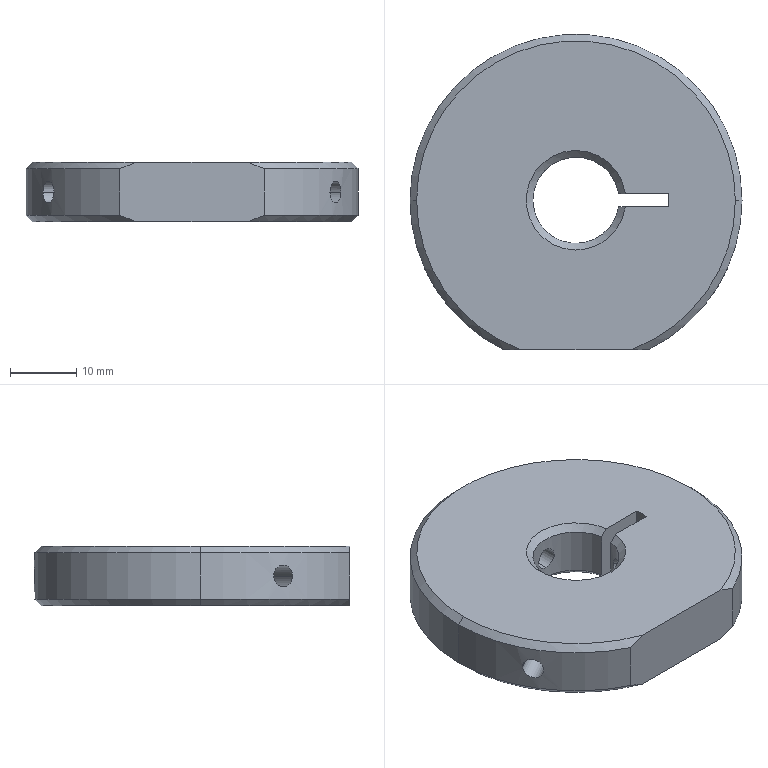Part | STEP file | 11-FG-B05911 | 1 solid | 26 faces | box 50 x 47.5 x 9 mm | volume 15360 mm3 | cylinder 12 | cone 9 | plane 5 | commonest cylinder face diameters 3.3 x6 50 x3 13 x2 28 x1
STEP:
#1=CARTESIAN_POINT('',(24.,0.,9.));
#2=VERTEX_POINT('',#1);
#3=CARTESIAN_POINT('',(-24.,0.,9.));
#4=VERTEX_POINT('',#3);
#5=CARTESIAN_POINT('',(0.,0.,9.));
#6=DIRECTION('',(0.,0.,1.));
#7=DIRECTION('',(1.,0.,0.));
#8=AXIS2_PLACEMENT_3D('',#5,#6,#7);
#9=CIRCLE('',#8,24.);
#10=EDGE_CURVE('',#2,#4,#9,.T.);
#11=ORIENTED_EDGE('',*,*,#10,.F.);
#12=CARTESIAN_POINT('',(25.,0.,8.));
#13=VERTEX_POINT('',#12);
#14=CARTESIAN_POINT('',(24.,0.,9.));
#15=DIRECTION('',(0.7071,0.,-0.7071));
#16=VECTOR('',#15,1000.);
#17=LINE('',#14,#16);
#18=EDGE_CURVE('',#2,#13,#17,.T.);
#19=ORIENTED_EDGE('',*,*,#18,.T.);
#20=CARTESIAN_POINT('',(-25.,0.,8.));
#21=VERTEX_POINT('',#20);
#22=CARTESIAN_POINT('',(0.,0.,8.));
#23=DIRECTION('',(0.,0.,-1.));
#24=DIRECTION('',(1.,0.,0.));
#25=AXIS2_PLACEMENT_3D('',#22,#23,#24);
#26=CIRCLE('',#25,25.);
#27=EDGE_CURVE('',#21,#13,#26,.T.);
#28=ORIENTED_EDGE('',*,*,#27,.F.);
#29=CARTESIAN_POINT('',(-24.,0.,9.));
#30=DIRECTION('',(-0.7071,0.,-0.7071));
#31=VECTOR('',#30,1000.);
#32=LINE('',#29,#31);
#33=EDGE_CURVE('',#4,#21,#32,.T.);
#34=ORIENTED_EDGE('',*,*,#33,.F.);
#35=EDGE_LOOP('',(#11,#19,#28,#34));
#36=FACE_OUTER_BOUND('',#35,.T.);
#37=CARTESIAN_POINT('',(0.,0.,9.));
#38=DIRECTION('',(0.,0.,-1.));
#39=DIRECTION('',(-1.,0.,0.));
#40=AXIS2_PLACEMENT_3D('',#37,#38,#39);
#41=CONICAL_SURFACE('',#40,24.,0.7854);
#42=ADVANCED_FACE('',(#36),#41,.T.);
#43=CARTESIAN_POINT('',(-8.352,-22.5,9.));
#44=VERTEX_POINT('',#43);
#45=CARTESIAN_POINT('',(0.,0.,9.));
#46=DIRECTION('',(0.,0.,1.));
#47=DIRECTION('',(1.,0.,0.));
#48=AXIS2_PLACEMENT_3D('',#45,#46,#47);
#49=CIRCLE('',#48,24.);
#50=EDGE_CURVE('',#4,#44,#49,.T.);
#51=ORIENTED_EDGE('',*,*,#50,.F.);
#52=ORIENTED_EDGE('',*,*,#33,.T.);
#53=CARTESIAN_POINT('',(-10.897,-22.5,8.));
#54=VERTEX_POINT('',#53);
#55=CARTESIAN_POINT('',(0.,0.,8.));
#56=DIRECTION('',(0.,0.,-1.));
#57=DIRECTION('',(1.,0.,0.));
#58=AXIS2_PLACEMENT_3D('',#55,#56,#57);
#59=CIRCLE('',#58,25.);
#60=EDGE_CURVE('',#54,#21,#59,.T.);
#61=ORIENTED_EDGE('',*,*,#60,.F.);
#62=CARTESIAN_POINT('',(-8.352,-22.5,9.));
#63=CARTESIAN_POINT('',(-9.21,-22.5,8.701));
#64=CARTESIAN_POINT('',(-10.062,-22.5,8.364));
#65=CARTESIAN_POINT('',(-10.897,-22.5,8.));
#66=B_SPLINE_CURVE_WITH_KNOTS('',3,(#62,#63,#64,#65),.UNSPECIFIED.,.F.,.F.,(4,4),(0.06645,0.06918),.UNSPECIFIED.);
#67=EDGE_CURVE('',#44,#54,#66,.T.);
#68=ORIENTED_EDGE('',*,*,#67,.F.);
#69=EDGE_LOOP('',(#51,#52,#61,#68));
#70=FACE_OUTER_BOUND('',#69,.T.);
#71=CARTESIAN_POINT('',(0.,0.,9.));
#72=DIRECTION('',(0.,0.,-1.));
#73=DIRECTION('',(-1.,0.,0.));
#74=AXIS2_PLACEMENT_3D('',#71,#72,#73);
#75=CONICAL_SURFACE('',#74,24.,0.7854);
#76=ADVANCED_FACE('',(#70),#75,.T.);
#77=CARTESIAN_POINT('',(-24.,0.,0.));
#78=VERTEX_POINT('',#77);
#79=CARTESIAN_POINT('',(24.,0.,0.));
#80=VERTEX_POINT('',#79);
#81=CARTESIAN_POINT('',(0.,0.,0.));
#82=DIRECTION('',(0.,0.,-1.));
#83=DIRECTION('',(1.,0.,0.));
#84=AXIS2_PLACEMENT_3D('',#81,#82,#83);
#85=CIRCLE('',#84,24.);
#86=EDGE_CURVE('',#78,#80,#85,.T.);
#87=ORIENTED_EDGE('',*,*,#86,.F.);
#88=CARTESIAN_POINT('',(-25.,0.,1.));
#89=VERTEX_POINT('',#88);
#90=CARTESIAN_POINT('',(-25.,0.,1.));
#91=DIRECTION('',(-0.7071,0.,0.7071));
#92=VECTOR('',#91,1000.);
#93=LINE('',#90,#92);
#94=EDGE_CURVE('',#78,#89,#93,.T.);
#95=ORIENTED_EDGE('',*,*,#94,.T.);
#96=CARTESIAN_POINT('',(25.,0.,1.));
#97=VERTEX_POINT('',#96);
#98=CARTESIAN_POINT('',(0.,0.,1.));
#99=DIRECTION('',(0.,0.,1.));
#100=DIRECTION('',(1.,0.,0.));
#101=AXIS2_PLACEMENT_3D('',#98,#99,#100);
#102=CIRCLE('',#101,25.);
#103=EDGE_CURVE('',#97,#89,#102,.T.);
#104=ORIENTED_EDGE('',*,*,#103,.F.);
#105=CARTESIAN_POINT('',(25.,0.,1.));
#106=DIRECTION('',(0.7071,0.,0.7071));
#107=VECTOR('',#106,1000.);
#108=LINE('',#105,#107);
#109=EDGE_CURVE('',#80,#97,#108,.T.);
#110=ORIENTED_EDGE('',*,*,#109,.F.);
#111=EDGE_LOOP('',(#87,#95,#104,#110));
#112=FACE_OUTER_BOUND('',#111,.T.);
#113=CARTESIAN_POINT('',(0.,0.,1.));
#114=DIRECTION('',(0.,0.,1.));
#115=DIRECTION('',(1.,0.,0.));
#116=AXIS2_PLACEMENT_3D('',#113,#114,#115);
#117=CONICAL_SURFACE('',#116,25.,0.7854);
#118=ADVANCED_FACE('',(#112),#117,.T.);
#119=CARTESIAN_POINT('',(8.352,-22.5,0.));
#120=VERTEX_POINT('',#119);
#121=CARTESIAN_POINT('',(0.,0.,0.));
#122=DIRECTION('',(0.,0.,-1.));
#123=DIRECTION('',(1.,0.,0.));
#124=AXIS2_PLACEMENT_3D('',#121,#122,#123);
#125=CIRCLE('',#124,24.);
#126=EDGE_CURVE('',#80,#120,#125,.T.);
#127=ORIENTED_EDGE('',*,*,#126,.F.);
#128=ORIENTED_EDGE('',*,*,#109,.T.);
#129=CARTESIAN_POINT('',(10.897,-22.5,1.));
#130=VERTEX_POINT('',#129);
#131=CARTESIAN_POINT('',(0.,0.,1.));
#132=DIRECTION('',(0.,0.,1.));
#133=DIRECTION('',(1.,0.,0.));
#134=AXIS2_PLACEMENT_3D('',#131,#132,#133);
#135=CIRCLE('',#134,25.);
#136=EDGE_CURVE('',#130,#97,#135,.T.);
#137=ORIENTED_EDGE('',*,*,#136,.F.);
#138=CARTESIAN_POINT('',(8.352,-22.5,0.));
#139=CARTESIAN_POINT('',(9.21,-22.5,0.2988));
#140=CARTESIAN_POINT('',(10.062,-22.5,0.6359));
#141=CARTESIAN_POINT('',(10.897,-22.5,1.));
#142=B_SPLINE_CURVE_WITH_KNOTS('',3,(#138,#139,#140,#141),.UNSPECIFIED.,.F.,.F.,(4,4),(0.06645,0.06918),.UNSPECIFIED.);
#143=EDGE_CURVE('',#120,#130,#142,.T.);
#144=ORIENTED_EDGE('',*,*,#143,.F.);
#145=EDGE_LOOP('',(#127,#128,#137,#144));
#146=FACE_OUTER_BOUND('',#145,.T.);
#147=CARTESIAN_POINT('',(0.,0.,1.));
#148=DIRECTION('',(0.,0.,1.));
#149=DIRECTION('',(1.,0.,0.));
#150=AXIS2_PLACEMENT_3D('',#147,#148,#149);
#151=CONICAL_SURFACE('',#150,25.,0.7854);
#152=ADVANCED_FACE('',(#146),#151,.T.);
#153=CARTESIAN_POINT('',(-6.5,0.,1.));
#154=VERTEX_POINT('',#153);
#155=CARTESIAN_POINT('',(6.423,1.,1.));
#156=VERTEX_POINT('',#155);
#157=CARTESIAN_POINT('',(0.,0.,1.));
#158=DIRECTION('',(0.,0.,-1.));
#159=DIRECTION('',(1.,0.,0.));
#160=AXIS2_PLACEMENT_3D('',#157,#158,#159);
#161=CIRCLE('',#160,6.5);
#162=EDGE_CURVE('',#154,#156,#161,.T.);
#163=ORIENTED_EDGE('',*,*,#162,.F.);
#164=CARTESIAN_POINT('',(-7.5,0.,0.));
#165=VERTEX_POINT('',#164);
#166=CARTESIAN_POINT('',(-7.5,0.,0.));
#167=DIRECTION('',(-0.7071,0.,-0.7071));
#168=VECTOR('',#167,1000.);
#169=LINE('',#166,#168);
#170=EDGE_CURVE('',#154,#165,#169,.T.);
#171=ORIENTED_EDGE('',*,*,#170,.T.);
#172=CARTESIAN_POINT('',(7.433,1.,0.));
#173=VERTEX_POINT('',#172);
#174=CARTESIAN_POINT('',(0.,0.,0.));
#175=DIRECTION('',(0.,0.,1.));
#176=DIRECTION('',(1.,0.,0.));
#177=AXIS2_PLACEMENT_3D('',#174,#175,#176);
#178=CIRCLE('',#177,7.5);
#179=EDGE_CURVE('',#173,#165,#178,.T.);
#180=ORIENTED_EDGE('',*,*,#179,.F.);
#181=CARTESIAN_POINT('',(6.423,1.,1.));
#182=CARTESIAN_POINT('',(6.595,1.,0.8297));
#183=CARTESIAN_POINT('',(6.767,1.,0.6594));
#184=CARTESIAN_POINT('',(6.939,1.,0.4889));
#185=CARTESIAN_POINT('',(7.104,1.,0.326));
#186=CARTESIAN_POINT('',(7.269,1.,0.163));
#187=CARTESIAN_POINT('',(7.433,1.,0.));
#188=B_SPLINE_CURVE_WITH_KNOTS('',3,(#181,#182,#183,#184,#185,#186,#187),.UNSPECIFIED.,.F.,.F.,(4,3,4),(0.001962,0.002688,0.003383),.UNSPECIFIED.);
#189=EDGE_CURVE('',#156,#173,#188,.T.);
#190=ORIENTED_EDGE('',*,*,#189,.F.);
#191=EDGE_LOOP('',(#163,#171,#180,#190));
#192=FACE_OUTER_BOUND('',#191,.T.);
#193=CARTESIAN_POINT('',(0.,0.,0.));
#194=DIRECTION('',(0.,0.,-1.));
#195=DIRECTION('',(-1.,0.,0.));
#196=AXIS2_PLACEMENT_3D('',#193,#194,#195);
#197=CONICAL_SURFACE('',#196,7.5,0.7854);
#198=ADVANCED_FACE('',(#192),#197,.F.);
#199=CARTESIAN_POINT('',(-20.778,-13.902,4.5));
#200=VERTEX_POINT('',#199);
#201=CARTESIAN_POINT('',(-22.428,-11.044,4.5));
#202=VERTEX_POINT('',#201);
#203=CARTESIAN_POINT('',(-20.778,-13.902,4.5));
#204=CARTESIAN_POINT('',(-20.778,-13.902,4.285));
#205=CARTESIAN_POINT('',(-20.803,-13.866,4.068));
#206=CARTESIAN_POINT('',(-20.893,-13.728,3.67));
#207=CARTESIAN_POINT('',(-20.961,-13.626,3.486));
#208=CARTESIAN_POINT('',(-21.084,-13.433,3.258));
#209=CARTESIAN_POINT('',(-21.13,-13.362,3.188));
#210=CARTESIAN_POINT('',(-21.225,-13.21,3.068));
#211=CARTESIAN_POINT('',(-21.275,-13.129,3.018));
#212=CARTESIAN_POINT('',(-21.379,-12.959,2.935));
#213=CARTESIAN_POINT('',(-21.434,-12.869,2.903));
#214=CARTESIAN_POINT('',(-21.541,-12.688,2.861));
#215=CARTESIAN_POINT('',(-21.596,-12.595,2.85));
#216=CARTESIAN_POINT('',(-21.759,-12.313,2.85));
#217=CARTESIAN_POINT('',(-21.863,-12.126,2.893));
#218=CARTESIAN_POINT('',(-22.007,-11.862,3.017));
#219=CARTESIAN_POINT('',(-22.052,-11.778,3.067));
#220=CARTESIAN_POINT('',(-22.136,-11.62,3.187));
#221=CARTESIAN_POINT('',(-22.175,-11.544,3.256));
#222=CARTESIAN_POINT('',(-22.28,-11.341,3.485));
#223=CARTESIAN_POINT('',(-22.335,-11.231,3.668));
#224=CARTESIAN_POINT('',(-22.409,-11.083,4.065));
#225=CARTESIAN_POINT('',(-22.428,-11.044,4.282));
#226=CARTESIAN_POINT('',(-22.428,-11.044,4.5));
#227=B_SPLINE_CURVE_WITH_KNOTS('',3,(#203,#204,#205,#206,#207,#208,#209,#210,#211,#212,#213,#214,#215,#216,#217,#218,#219,#220,#221,#222,#223,#224,#225,#226),.UNSPECIFIED.,.F.,.F.,(4,2,2,2,2,2,2,2,2,2,2,4),(0.00516,0.005805,0.00645,0.006772,0.007095,0.007417,0.007739,0.008384,0.008707,0.009029,0.009674,0.01032),.UNSPECIFIED.);
#228=EDGE_CURVE('',#200,#202,#227,.T.);
#229=ORIENTED_EDGE('',*,*,#228,.F.);
#230=CARTESIAN_POINT('',(-4.62,-4.572,4.5));
#231=VERTEX_POINT('',#230);
#232=CARTESIAN_POINT('',(0.825,-1.429,4.5));
#233=DIRECTION('',(0.866,0.5,0.));
#234=VECTOR('',#233,1000.);
#235=LINE('',#232,#234);
#236=EDGE_CURVE('',#200,#231,#235,.T.);
#237=ORIENTED_EDGE('',*,*,#236,.T.);
#238=CARTESIAN_POINT('',(-6.27,-1.715,4.5));
#239=VERTEX_POINT('',#238);
#240=CARTESIAN_POINT('',(-4.62,-4.572,4.5));
#241=CARTESIAN_POINT('',(-4.62,-4.572,4.284));
#242=CARTESIAN_POINT('',(-4.652,-4.541,4.066));
#243=CARTESIAN_POINT('',(-4.74,-4.448,3.768));
#244=CARTESIAN_POINT('',(-4.776,-4.41,3.672));
#245=CARTESIAN_POINT('',(-4.858,-4.319,3.493));
#246=CARTESIAN_POINT('',(-4.904,-4.267,3.41));
#247=CARTESIAN_POINT('',(-5.004,-4.149,3.258));
#248=CARTESIAN_POINT('',(-5.058,-4.083,3.188));
#249=CARTESIAN_POINT('',(-5.169,-3.941,3.069));
#250=CARTESIAN_POINT('',(-5.227,-3.865,3.018));
#251=CARTESIAN_POINT('',(-5.403,-3.619,2.893));
#252=CARTESIAN_POINT('',(-5.52,-3.439,2.85));
#253=CARTESIAN_POINT('',(-5.683,-3.156,2.85));
#254=CARTESIAN_POINT('',(-5.735,-3.062,2.861));
#255=CARTESIAN_POINT('',(-5.832,-2.873,2.903));
#256=CARTESIAN_POINT('',(-5.877,-2.778,2.935));
#257=CARTESIAN_POINT('',(-6.001,-2.505,3.059));
#258=CARTESIAN_POINT('',(-6.069,-2.332,3.181));
#259=CARTESIAN_POINT('',(-6.173,-2.042,3.484));
#260=CARTESIAN_POINT('',(-6.21,-1.922,3.667));
#261=CARTESIAN_POINT('',(-6.246,-1.8,3.965));
#262=CARTESIAN_POINT('',(-6.255,-1.768,4.07));
#263=CARTESIAN_POINT('',(-6.267,-1.725,4.283));
#264=CARTESIAN_POINT('',(-6.27,-1.715,4.391));
#265=CARTESIAN_POINT('',(-6.27,-1.715,4.5));
#266=B_SPLINE_CURVE_WITH_KNOTS('',3,(#240,#241,#242,#243,#244,#245,#246,#247,#248,#249,#250,#251,#252,#253,#254,#255,#256,#257,#258,#259,#260,#261,#262,#263,#264,#265),.UNSPECIFIED.,.F.,.F.,(4,2,2,2,2,2,2,2,2,2,2,2,4),(0.00518,0.005827,0.006151,0.006474,0.006798,0.007122,0.007769,0.008093,0.008416,0.009064,0.009711,0.01003,0.01036),.UNSPECIFIED.);
#267=EDGE_CURVE('',#231,#239,#266,.T.);
#268=ORIENTED_EDGE('',*,*,#267,.T.);
#269=CARTESIAN_POINT('',(-0.825,1.429,4.5));
#270=DIRECTION('',(0.866,0.5,0.));
#271=VECTOR('',#270,1000.);
#272=LINE('',#269,#271);
#273=EDGE_CURVE('',#202,#239,#272,.T.);
#274=ORIENTED_EDGE('',*,*,#273,.F.);
#275=EDGE_LOOP('',(#229,#237,#268,#274));
#276=FACE_OUTER_BOUND('',#275,.T.);
#277=CARTESIAN_POINT('',(0.,0.,4.5));
#278=DIRECTION('',(0.866,0.5,0.));
#279=DIRECTION('',(-0.5,0.866,0.));
#280=AXIS2_PLACEMENT_3D('',#277,#278,#279);
#281=CYLINDRICAL_SURFACE('',#280,1.65);
#282=ADVANCED_FACE('',(#276),#281,.F.);
#283=CARTESIAN_POINT('',(22.428,-11.044,4.5));
#284=VERTEX_POINT('',#283);
#285=CARTESIAN_POINT('',(20.778,-13.902,4.5));
#286=VERTEX_POINT('',#285);
#287=CARTESIAN_POINT('',(22.428,-11.044,4.5));
#288=CARTESIAN_POINT('',(22.428,-11.044,4.285));
#289=CARTESIAN_POINT('',(22.409,-11.083,4.068));
#290=CARTESIAN_POINT('',(22.336,-11.23,3.67));
#291=CARTESIAN_POINT('',(22.281,-11.34,3.486));
#292=CARTESIAN_POINT('',(22.176,-11.543,3.258));
#293=CARTESIAN_POINT('',(22.137,-11.618,3.188));
#294=CARTESIAN_POINT('',(22.053,-11.777,3.068));
#295=CARTESIAN_POINT('',(22.008,-11.86,3.018));
#296=CARTESIAN_POINT('',(21.912,-12.036,2.935));
#297=CARTESIAN_POINT('',(21.862,-12.127,2.903));
#298=CARTESIAN_POINT('',(21.759,-12.311,2.861));
#299=CARTESIAN_POINT('',(21.706,-12.405,2.85));
#300=CARTESIAN_POINT('',(21.542,-12.687,2.85));
#301=CARTESIAN_POINT('',(21.433,-12.871,2.893));
#302=CARTESIAN_POINT('',(21.276,-13.128,3.017));
#303=CARTESIAN_POINT('',(21.226,-13.208,3.067));
#304=CARTESIAN_POINT('',(21.131,-13.36,3.187));
#305=CARTESIAN_POINT('',(21.085,-13.432,3.256));
#306=CARTESIAN_POINT('',(20.962,-13.624,3.485));
#307=CARTESIAN_POINT('',(20.894,-13.727,3.668));
#308=CARTESIAN_POINT('',(20.803,-13.865,4.065));
#309=CARTESIAN_POINT('',(20.778,-13.902,4.282));
#310=CARTESIAN_POINT('',(20.778,-13.902,4.5));
#311=B_SPLINE_CURVE_WITH_KNOTS('',3,(#287,#288,#289,#290,#291,#292,#293,#294,#295,#296,#297,#298,#299,#300,#301,#302,#303,#304,#305,#306,#307,#308,#309,#310),.UNSPECIFIED.,.F.,.F.,(4,2,2,2,2,2,2,2,2,2,2,4),(0.00516,0.005805,0.00645,0.006772,0.007095,0.007417,0.007739,0.008384,0.008707,0.009029,0.009674,0.01032),.UNSPECIFIED.);
#312=EDGE_CURVE('',#284,#286,#311,.T.);
#313=ORIENTED_EDGE('',*,*,#312,.F.);
#314=CARTESIAN_POINT('',(6.27,-1.715,4.5));
#315=VERTEX_POINT('',#314);
#316=CARTESIAN_POINT('',(0.825,1.429,4.5));
#317=DIRECTION('',(-0.866,0.5,0.));
#318=VECTOR('',#317,1000.);
#319=LINE('',#316,#318);
#320=EDGE_CURVE('',#284,#315,#319,.T.);
#321=ORIENTED_EDGE('',*,*,#320,.T.);
#322=CARTESIAN_POINT('',(4.62,-4.572,4.5));
#323=VERTEX_POINT('',#322);
#324=CARTESIAN_POINT('',(6.27,-1.715,4.5));
#325=CARTESIAN_POINT('',(6.27,-1.715,4.284));
#326=CARTESIAN_POINT('',(6.258,-1.758,4.066));
#327=CARTESIAN_POINT('',(6.222,-1.88,3.768));
#328=CARTESIAN_POINT('',(6.207,-1.931,3.672));
#329=CARTESIAN_POINT('',(6.169,-2.048,3.493));
#330=CARTESIAN_POINT('',(6.147,-2.113,3.41));
#331=CARTESIAN_POINT('',(6.095,-2.259,3.258));
#332=CARTESIAN_POINT('',(6.065,-2.339,3.188));
#333=CARTESIAN_POINT('',(5.998,-2.506,3.069));
#334=CARTESIAN_POINT('',(5.961,-2.594,3.018));
#335=CARTESIAN_POINT('',(5.836,-2.869,2.893));
#336=CARTESIAN_POINT('',(5.738,-3.061,2.85));
#337=CARTESIAN_POINT('',(5.575,-3.344,2.85));
#338=CARTESIAN_POINT('',(5.519,-3.435,2.861));
#339=CARTESIAN_POINT('',(5.404,-3.614,2.903));
#340=CARTESIAN_POINT('',(5.344,-3.701,2.935));
#341=CARTESIAN_POINT('',(5.17,-3.945,3.059));
#342=CARTESIAN_POINT('',(5.054,-4.09,3.181));
#343=CARTESIAN_POINT('',(4.855,-4.325,3.484));
#344=CARTESIAN_POINT('',(4.769,-4.417,3.667));
#345=CARTESIAN_POINT('',(4.682,-4.509,3.965));
#346=CARTESIAN_POINT('',(4.658,-4.533,4.07));
#347=CARTESIAN_POINT('',(4.628,-4.565,4.283));
#348=CARTESIAN_POINT('',(4.62,-4.572,4.391));
#349=CARTESIAN_POINT('',(4.62,-4.572,4.5));
#350=B_SPLINE_CURVE_WITH_KNOTS('',3,(#324,#325,#326,#327,#328,#329,#330,#331,#332,#333,#334,#335,#336,#337,#338,#339,#340,#341,#342,#343,#344,#345,#346,#347,#348,#349),.UNSPECIFIED.,.F.,.F.,(4,2,2,2,2,2,2,2,2,2,2,2,4),(0.00518,0.005827,0.006151,0.006474,0.006798,0.007122,0.007769,0.008093,0.008416,0.009064,0.009711,0.01003,0.01036),.UNSPECIFIED.);
#351=EDGE_CURVE('',#315,#323,#350,.T.);
#352=ORIENTED_EDGE('',*,*,#351,.T.);
#353=CARTESIAN_POINT('',(-0.825,-1.429,4.5));
#354=DIRECTION('',(-0.866,0.5,0.));
#355=VECTOR('',#354,1000.);
#356=LINE('',#353,#355);
#357=EDGE_CURVE('',#286,#323,#356,.T.);
#358=ORIENTED_EDGE('',*,*,#357,.F.);
#359=EDGE_LOOP('',(#313,#321,#352,#358));
#360=FACE_OUTER_BOUND('',#359,.T.);
#361=CARTESIAN_POINT('',(0.,0.,4.5));
#362=DIRECTION('',(-0.866,0.5,0.));
#363=DIRECTION('',(-0.5,-0.866,0.));
#364=AXIS2_PLACEMENT_3D('',#361,#362,#363);
#365=CYLINDRICAL_SURFACE('',#364,1.65);
#366=ADVANCED_FACE('',(#360),#365,.F.);
#367=CARTESIAN_POINT('',(0.,25.,6.15));
#368=VERTEX_POINT('',#367);
#369=CARTESIAN_POINT('',(0.,25.,2.85));
#370=VERTEX_POINT('',#369);
#371=CARTESIAN_POINT('',(0.,25.,6.15));
#372=CARTESIAN_POINT('',(-0.2154,25.,6.15));
#373=CARTESIAN_POINT('',(-0.4324,24.997,6.107));
#374=CARTESIAN_POINT('',(-0.8296,24.987,5.942));
#375=CARTESIAN_POINT('',(-1.014,24.98,5.82));
#376=CARTESIAN_POINT('',(-1.242,24.969,5.592));
#377=CARTESIAN_POINT('',(-1.312,24.966,5.507));
#378=CARTESIAN_POINT('',(-1.432,24.959,5.327));
#379=CARTESIAN_POINT('',(-1.482,24.956,5.233));
#380=CARTESIAN_POINT('',(-1.565,24.951,5.033));
#381=CARTESIAN_POINT('',(-1.597,24.949,4.928));
#382=CARTESIAN_POINT('',(-1.639,24.946,4.717));
#383=CARTESIAN_POINT('',(-1.65,24.945,4.61));
#384=CARTESIAN_POINT('',(-1.65,24.945,4.284));
#385=CARTESIAN_POINT('',(-1.607,24.948,4.069));
#386=CARTESIAN_POINT('',(-1.483,24.956,3.769));
#387=CARTESIAN_POINT('',(-1.433,24.959,3.675));
#388=CARTESIAN_POINT('',(-1.313,24.966,3.495));
#389=CARTESIAN_POINT('',(-1.244,24.969,3.41));
#390=CARTESIAN_POINT('',(-1.015,24.98,3.182));
#391=CARTESIAN_POINT('',(-0.8316,24.987,3.059));
#392=CARTESIAN_POINT('',(-0.4347,24.997,2.894));
#393=CARTESIAN_POINT('',(-0.2181,25.,2.85));
#394=CARTESIAN_POINT('',(0.,25.,2.85));
#395=B_SPLINE_CURVE_WITH_KNOTS('',3,(#371,#372,#373,#374,#375,#376,#377,#378,#379,#380,#381,#382,#383,#384,#385,#386,#387,#388,#389,#390,#391,#392,#393,#394),.UNSPECIFIED.,.F.,.F.,(4,2,2,2,2,2,2,2,2,2,2,4),(0.00516,0.005805,0.00645,0.006772,0.007095,0.007417,0.007739,0.008384,0.008707,0.009029,0.009674,0.01032),.UNSPECIFIED.);
#396=EDGE_CURVE('',#368,#370,#395,.T.);
#397=ORIENTED_EDGE('',*,*,#396,.F.);
#398=CARTESIAN_POINT('',(0.,6.5,6.15));
#399=VERTEX_POINT('',#398);
#400=CARTESIAN_POINT('',(0.,0.,6.15));
#401=DIRECTION('',(0.,-1.,0.));
#402=VECTOR('',#401,1000.);
#403=LINE('',#400,#402);
#404=EDGE_CURVE('',#368,#399,#403,.T.);
#405=ORIENTED_EDGE('',*,*,#404,.T.);
#406=CARTESIAN_POINT('',(0.,6.5,2.85));
#407=VERTEX_POINT('',#406);
#408=CARTESIAN_POINT('',(0.,6.5,6.15));
#409=CARTESIAN_POINT('',(-0.2158,6.5,6.15));
#410=CARTESIAN_POINT('',(-0.4338,6.489,6.106));
#411=CARTESIAN_POINT('',(-0.7319,6.459,5.983));
#412=CARTESIAN_POINT('',(-0.8284,6.448,5.931));
#413=CARTESIAN_POINT('',(-1.007,6.422,5.811));
#414=CARTESIAN_POINT('',(-1.09,6.408,5.743));
#415=CARTESIAN_POINT('',(-1.242,6.381,5.591));
#416=CARTESIAN_POINT('',(-1.312,6.367,5.507));
#417=CARTESIAN_POINT('',(-1.431,6.341,5.329));
#418=CARTESIAN_POINT('',(-1.482,6.329,5.234));
#419=CARTESIAN_POINT('',(-1.607,6.299,4.933));
#420=CARTESIAN_POINT('',(-1.65,6.287,4.718));
#421=CARTESIAN_POINT('',(-1.65,6.287,4.392));
#422=CARTESIAN_POINT('',(-1.639,6.29,4.284));
#423=CARTESIAN_POINT('',(-1.597,6.301,4.072));
#424=CARTESIAN_POINT('',(-1.565,6.309,3.967));
#425=CARTESIAN_POINT('',(-1.441,6.339,3.669));
#426=CARTESIAN_POINT('',(-1.319,6.367,3.485));
#427=CARTESIAN_POINT('',(-1.016,6.422,3.182));
#428=CARTESIAN_POINT('',(-0.833,6.449,3.06));
#429=CARTESIAN_POINT('',(-0.5351,6.479,2.935));
#430=CARTESIAN_POINT('',(-0.43,6.487,2.903));
#431=CARTESIAN_POINT('',(-0.2173,6.497,2.861));
#432=CARTESIAN_POINT('',(-0.1095,6.5,2.85));
#433=CARTESIAN_POINT('',(0.,6.5,2.85));
#434=B_SPLINE_CURVE_WITH_KNOTS('',3,(#408,#409,#410,#411,#412,#413,#414,#415,#416,#417,#418,#419,#420,#421,#422,#423,#424,#425,#426,#427,#428,#429,#430,#431,#432,#433),.UNSPECIFIED.,.F.,.F.,(4,2,2,2,2,2,2,2,2,2,2,2,4),(0.00518,0.005827,0.006151,0.006475,0.006798,0.007122,0.007769,0.008093,0.008416,0.009064,0.009711,0.01003,0.01036),.UNSPECIFIED.);
#435=EDGE_CURVE('',#399,#407,#434,.T.);
#436=ORIENTED_EDGE('',*,*,#435,.T.);
#437=CARTESIAN_POINT('',(0.,0.,2.85));
#438=DIRECTION('',(0.,-1.,0.));
#439=VECTOR('',#438,1000.);
#440=LINE('',#437,#439);
#441=EDGE_CURVE('',#370,#407,#440,.T.);
#442=ORIENTED_EDGE('',*,*,#441,.F.);
#443=EDGE_LOOP('',(#397,#405,#436,#442));
#444=FACE_OUTER_BOUND('',#443,.T.);
#445=CARTESIAN_POINT('',(0.,0.,4.5));
#446=DIRECTION('',(0.,-1.,0.));
#447=DIRECTION('',(0.,0.,-1.));
#448=AXIS2_PLACEMENT_3D('',#445,#446,#447);
#449=CYLINDRICAL_SURFACE('',#448,1.65);
#450=ADVANCED_FACE('',(#444),#449,.F.);
#451=CARTESIAN_POINT('',(0.,6.5,2.85));
#452=CARTESIAN_POINT('',(0.1095,6.5,2.85));
#453=CARTESIAN_POINT('',(0.2171,6.497,2.861));
#454=CARTESIAN_POINT('',(0.4286,6.487,2.903));
#455=CARTESIAN_POINT('',(0.5337,6.479,2.935));
#456=CARTESIAN_POINT('',(0.7333,6.459,3.018));
#457=CARTESIAN_POINT('',(0.8279,6.448,3.069));
#458=CARTESIAN_POINT('',(1.007,6.422,3.188));
#459=CARTESIAN_POINT('',(1.091,6.408,3.258));
#460=CARTESIAN_POINT('',(1.319,6.367,3.485));
#461=CARTESIAN_POINT('',(1.441,6.339,3.669));
#462=CARTESIAN_POINT('',(1.606,6.299,4.065));
#463=CARTESIAN_POINT('',(1.65,6.287,4.283));
#464=CARTESIAN_POINT('',(1.65,6.287,4.607));
#465=CARTESIAN_POINT('',(1.639,6.29,4.717));
#466=CARTESIAN_POINT('',(1.597,6.301,4.929));
#467=CARTESIAN_POINT('',(1.566,6.309,5.032));
#468=CARTESIAN_POINT('',(1.441,6.339,5.333));
#469=CARTESIAN_POINT('',(1.319,6.367,5.514));
#470=CARTESIAN_POINT('',(1.09,6.408,5.743));
#471=CARTESIAN_POINT('',(1.007,6.422,5.811));
#472=CARTESIAN_POINT('',(0.8288,6.448,5.931));
#473=CARTESIAN_POINT('',(0.7321,6.459,5.983));
#474=CARTESIAN_POINT('',(0.533,6.479,6.065));
#475=CARTESIAN_POINT('',(0.4301,6.487,6.097));
#476=CARTESIAN_POINT('',(0.2175,6.497,6.139));
#477=CARTESIAN_POINT('',(0.108,6.5,6.15));
#478=CARTESIAN_POINT('',(0.,6.5,6.15));
#479=B_SPLINE_CURVE_WITH_KNOTS('',3,(#451,#452,#453,#454,#455,#456,#457,#458,#459,#460,#461,#462,#463,#464,#465,#466,#467,#468,#469,#470,#471,#472,#473,#474,#475,#476,#477,#478),.UNSPECIFIED.,.F.,.F.,(4,2,2,2,2,2,2,2,2,2,2,2,2,4),(0.,0.0003237,0.0006475,0.0009712,0.001295,0.001942,0.00259,0.002914,0.003237,0.003885,0.004209,0.004532,0.004856,0.00518),.UNSPECIFIED.);
#480=EDGE_CURVE('',#407,#399,#479,.T.);
#481=ORIENTED_EDGE('',*,*,#480,.F.);
#482=ORIENTED_EDGE('',*,*,#435,.F.);
#483=EDGE_LOOP('',(#481,#482));
#484=FACE_BOUND('',#483,.T.);
#485=CARTESIAN_POINT('',(6.423,1.,8.));
#486=VERTEX_POINT('',#485);
#487=CARTESIAN_POINT('',(-6.5,0.,8.));
#488=VERTEX_POINT('',#487);
#489=CARTESIAN_POINT('',(0.,0.,8.));
#490=DIRECTION('',(0.,0.,1.));
#491=DIRECTION('',(1.,0.,0.));
#492=AXIS2_PLACEMENT_3D('',#489,#490,#491);
#493=CIRCLE('',#492,6.5);
#494=EDGE_CURVE('',#486,#488,#493,.T.);
#495=ORIENTED_EDGE('',*,*,#494,.T.);
#496=CARTESIAN_POINT('',(-6.5,0.,9.));
#497=DIRECTION('',(0.,0.,-1.));
#498=VECTOR('',#497,1000.);
#499=LINE('',#496,#498);
#500=EDGE_CURVE('',#488,#154,#499,.T.);
#501=ORIENTED_EDGE('',*,*,#500,.T.);
#502=ORIENTED_EDGE('',*,*,#162,.T.);
#503=CARTESIAN_POINT('',(6.423,1.,19.));
#504=DIRECTION('',(0.,0.,-1.));
#505=VECTOR('',#504,1000.);
#506=LINE('',#503,#505);
#507=EDGE_CURVE('',#486,#156,#506,.T.);
#508=ORIENTED_EDGE('',*,*,#507,.F.);
#509=EDGE_LOOP('',(#495,#501,#502,#508));
#510=FACE_OUTER_BOUND('',#509,.T.);
#511=CARTESIAN_POINT('',(0.,0.,9.));
#512=DIRECTION('',(0.,0.,-1.));
#513=DIRECTION('',(-1.,0.,0.));
#514=AXIS2_PLACEMENT_3D('',#511,#512,#513);
#515=CYLINDRICAL_SURFACE('',#514,6.5);
#516=ADVANCED_FACE('',(#484,#510),#515,.F.);
#517=CARTESIAN_POINT('',(0.,25.,2.85));
#518=CARTESIAN_POINT('',(0.1091,25.,2.85));
#519=CARTESIAN_POINT('',(0.2163,24.999,2.861));
#520=CARTESIAN_POINT('',(0.4272,24.997,2.903));
#521=CARTESIAN_POINT('',(0.532,24.995,2.934));
#522=CARTESIAN_POINT('',(0.7318,24.989,3.017));
#523=CARTESIAN_POINT('',(0.8266,24.986,3.068));
#524=CARTESIAN_POINT('',(1.006,24.98,3.188));
#525=CARTESIAN_POINT('',(1.091,24.976,3.257));
#526=CARTESIAN_POINT('',(1.319,24.966,3.486));
#527=CARTESIAN_POINT('',(1.442,24.959,3.67));
#528=CARTESIAN_POINT('',(1.607,24.948,4.067));
#529=CARTESIAN_POINT('',(1.65,24.945,4.284));
#530=CARTESIAN_POINT('',(1.65,24.945,4.607));
#531=CARTESIAN_POINT('',(1.639,24.946,4.716));
#532=CARTESIAN_POINT('',(1.597,24.949,4.928));
#533=CARTESIAN_POINT('',(1.566,24.951,5.031));
#534=CARTESIAN_POINT('',(1.483,24.956,5.231));
#535=CARTESIAN_POINT('',(1.432,24.959,5.327));
#536=CARTESIAN_POINT('',(1.312,24.966,5.506));
#537=CARTESIAN_POINT('',(1.244,24.969,5.589));
#538=CARTESIAN_POINT('',(1.09,24.976,5.744));
#539=CARTESIAN_POINT('',(1.007,24.98,5.812));
#540=CARTESIAN_POINT('',(0.8278,24.986,5.931));
#541=CARTESIAN_POINT('',(0.7314,24.989,5.983));
#542=CARTESIAN_POINT('',(0.5314,24.995,6.066));
#543=CARTESIAN_POINT('',(0.4286,24.997,6.097));
#544=CARTESIAN_POINT('',(0.2171,24.999,6.139));
#545=CARTESIAN_POINT('',(0.1077,25.,6.15));
#546=CARTESIAN_POINT('',(0.,25.,6.15));
#547=B_SPLINE_CURVE_WITH_KNOTS('',3,(#517,#518,#519,#520,#521,#522,#523,#524,#525,#526,#527,#528,#529,#530,#531,#532,#533,#534,#535,#536,#537,#538,#539,#540,#541,#542,#543,#544,#545,#546),.UNSPECIFIED.,.F.,.F.,(4,2,2,2,2,2,2,2,2,2,2,2,2,2,4),(0.,0.0003225,0.000645,0.0009675,0.00129,0.001935,0.00258,0.002903,0.003225,0.003548,0.00387,0.004193,0.004515,0.004838,0.00516),.UNSPECIFIED.);
#548=EDGE_CURVE('',#370,#368,#547,.T.);
#549=ORIENTED_EDGE('',*,*,#548,.T.);
#550=ORIENTED_EDGE('',*,*,#396,.T.);
#551=EDGE_LOOP('',(#549,#550));
#552=FACE_BOUND('',#551,.T.);
#553=ORIENTED_EDGE('',*,*,#27,.T.);
#554=CARTESIAN_POINT('',(25.,0.,9.));
#555=DIRECTION('',(0.,0.,-1.));
#556=VECTOR('',#555,1000.);
#557=LINE('',#554,#556);
#558=EDGE_CURVE('',#13,#97,#557,.T.);
#559=ORIENTED_EDGE('',*,*,#558,.T.);
#560=ORIENTED_EDGE('',*,*,#103,.T.);
#561=CARTESIAN_POINT('',(-25.,0.,9.));
#562=DIRECTION('',(0.,0.,-1.));
#563=VECTOR('',#562,1000.);
#564=LINE('',#561,#563);
#565=EDGE_CURVE('',#21,#89,#564,.T.);
#566=ORIENTED_EDGE('',*,*,#565,.F.);
#567=EDGE_LOOP('',(#553,#559,#560,#566));
#568=FACE_OUTER_BOUND('',#567,.T.);
#569=CARTESIAN_POINT('',(0.,0.,9.));
#570=DIRECTION('',(0.,0.,-1.));
#571=DIRECTION('',(-1.,0.,0.));
#572=AXIS2_PLACEMENT_3D('',#569,#570,#571);
#573=CYLINDRICAL_SURFACE('',#572,25.);
#574=ADVANCED_FACE('',(#552,#568),#573,.T.);
#575=CARTESIAN_POINT('',(-22.428,-11.044,4.5));
#576=CARTESIAN_POINT('',(-22.428,-11.044,4.609));
#577=CARTESIAN_POINT('',(-22.424,-11.053,4.716));
#578=CARTESIAN_POINT('',(-22.405,-11.091,4.927));
#579=CARTESIAN_POINT('',(-22.391,-11.12,5.032));
#580=CARTESIAN_POINT('',(-22.354,-11.194,5.232));
#581=CARTESIAN_POINT('',(-22.331,-11.239,5.327));
#582=CARTESIAN_POINT('',(-22.277,-11.346,5.506));
#583=CARTESIAN_POINT('',(-22.245,-11.408,5.591));
#584=CARTESIAN_POINT('',(-22.14,-11.612,5.819));
#585=CARTESIAN_POINT('',(-22.054,-11.775,5.942));
#586=CARTESIAN_POINT('',(-21.865,-12.123,6.107));
#587=CARTESIAN_POINT('',(-21.759,-12.313,6.15));
#588=CARTESIAN_POINT('',(-21.597,-12.593,6.15));
#589=CARTESIAN_POINT('',(-21.542,-12.687,6.139));
#590=CARTESIAN_POINT('',(-21.434,-12.869,6.097));
#591=CARTESIAN_POINT('',(-21.38,-12.957,6.066));
#592=CARTESIAN_POINT('',(-21.276,-13.128,5.983));
#593=CARTESIAN_POINT('',(-21.225,-13.21,5.932));
#594=CARTESIAN_POINT('',(-21.13,-13.361,5.812));
#595=CARTESIAN_POINT('',(-21.085,-13.432,5.744));
#596=CARTESIAN_POINT('',(-21.002,-13.562,5.59));
#597=CARTESIAN_POINT('',(-20.965,-13.619,5.507));
#598=CARTESIAN_POINT('',(-20.9,-13.719,5.328));
#599=CARTESIAN_POINT('',(-20.871,-13.762,5.231));
#600=CARTESIAN_POINT('',(-20.825,-13.832,5.031));
#601=CARTESIAN_POINT('',(-20.808,-13.858,4.929));
#602=CARTESIAN_POINT('',(-20.784,-13.893,4.717));
#603=CARTESIAN_POINT('',(-20.778,-13.902,4.608));
#604=CARTESIAN_POINT('',(-20.778,-13.902,4.5));
#605=B_SPLINE_CURVE_WITH_KNOTS('',3,(#575,#576,#577,#578,#579,#580,#581,#582,#583,#584,#585,#586,#587,#588,#589,#590,#591,#592,#593,#594,#595,#596,#597,#598,#599,#600,#601,#602,#603,#604),.UNSPECIFIED.,.F.,.F.,(4,2,2,2,2,2,2,2,2,2,2,2,2,2,4),(0.,0.0003225,0.000645,0.0009675,0.00129,0.001935,0.00258,0.002903,0.003225,0.003548,0.00387,0.004193,0.004515,0.004838,0.00516),.UNSPECIFIED.);
#606=EDGE_CURVE('',#202,#200,#605,.T.);
#607=ORIENTED_EDGE('',*,*,#606,.T.);
#608=ORIENTED_EDGE('',*,*,#228,.T.);
#609=EDGE_LOOP('',(#607,#608));
#610=FACE_BOUND('',#609,.T.);
#611=ORIENTED_EDGE('',*,*,#60,.T.);
#612=ORIENTED_EDGE('',*,*,#565,.T.);
#613=CARTESIAN_POINT('',(-10.897,-22.5,1.));
#614=VERTEX_POINT('',#613);
#615=CARTESIAN_POINT('',(0.,0.,1.));
#616=DIRECTION('',(0.,0.,1.));
#617=DIRECTION('',(1.,0.,0.));
#618=AXIS2_PLACEMENT_3D('',#615,#616,#617);
#619=CIRCLE('',#618,25.);
#620=EDGE_CURVE('',#89,#614,#619,.T.);
#621=ORIENTED_EDGE('',*,*,#620,.T.);
#622=CARTESIAN_POINT('',(-10.897,-22.5,9.));
#623=DIRECTION('',(0.,0.,1.));
#624=VECTOR('',#623,1000.);
#625=LINE('',#622,#624);
#626=EDGE_CURVE('',#614,#54,#625,.T.);
#627=ORIENTED_EDGE('',*,*,#626,.T.);
#628=EDGE_LOOP('',(#611,#612,#621,#627));
#629=FACE_OUTER_BOUND('',#628,.T.);
#630=CARTESIAN_POINT('',(0.,0.,9.));
#631=DIRECTION('',(0.,0.,-1.));
#632=DIRECTION('',(-1.,0.,0.));
#633=AXIS2_PLACEMENT_3D('',#630,#631,#632);
#634=CYLINDRICAL_SURFACE('',#633,25.);
#635=ADVANCED_FACE('',(#610,#629),#634,.T.);
#636=CARTESIAN_POINT('',(7.433,-1.,9.));
#637=VERTEX_POINT('',#636);
#638=CARTESIAN_POINT('',(13.964,-1.,9.));
#639=VERTEX_POINT('',#638);
#640=CARTESIAN_POINT('',(0.,-1.,9.));
#641=DIRECTION('',(1.,0.,0.));
#642=VECTOR('',#641,1000.);
#643=LINE('',#640,#642);
#644=EDGE_CURVE('',#637,#639,#643,.T.);
#645=ORIENTED_EDGE('',*,*,#644,.F.);
#646=CARTESIAN_POINT('',(7.433,1.,9.));
#647=VERTEX_POINT('',#646);
#648=CARTESIAN_POINT('',(0.,0.,9.));
#649=DIRECTION('',(0.,0.,-1.));
#650=DIRECTION('',(1.,0.,0.));
#651=AXIS2_PLACEMENT_3D('',#648,#649,#650);
#652=CIRCLE('',#651,7.5);
#653=EDGE_CURVE('',#637,#647,#652,.T.);
#654=ORIENTED_EDGE('',*,*,#653,.T.);
#655=CARTESIAN_POINT('',(13.964,1.,9.));
#656=VERTEX_POINT('',#655);
#657=CARTESIAN_POINT('',(0.,1.,9.));
#658=DIRECTION('',(-1.,0.,0.));
#659=VECTOR('',#658,1000.);
#660=LINE('',#657,#659);
#661=EDGE_CURVE('',#656,#647,#660,.T.);
#662=ORIENTED_EDGE('',*,*,#661,.F.);
#663=CARTESIAN_POINT('',(0.,0.,9.));
#664=DIRECTION('',(0.,0.,1.));
#665=DIRECTION('',(1.,0.,0.));
#666=AXIS2_PLACEMENT_3D('',#663,#664,#665);
#667=CIRCLE('',#666,14.);
#668=EDGE_CURVE('',#639,#656,#667,.T.);
#669=ORIENTED_EDGE('',*,*,#668,.F.);
#670=EDGE_LOOP('',(#645,#654,#662,#669));
#671=FACE_BOUND('',#670,.T.);
#672=CARTESIAN_POINT('',(8.352,-22.5,9.));
#673=VERTEX_POINT('',#672);
#674=CARTESIAN_POINT('',(-21.698,-22.5,9.));
#675=DIRECTION('',(-1.,0.,0.));
#676=VECTOR('',#675,1000.);
#677=LINE('',#674,#676);
#678=EDGE_CURVE('',#673,#44,#677,.T.);
#679=ORIENTED_EDGE('',*,*,#678,.F.);
#680=CARTESIAN_POINT('',(0.,0.,9.));
#681=DIRECTION('',(0.,0.,1.));
#682=DIRECTION('',(1.,0.,0.));
#683=AXIS2_PLACEMENT_3D('',#680,#681,#682);
#684=CIRCLE('',#683,24.);
#685=EDGE_CURVE('',#673,#2,#684,.T.);
#686=ORIENTED_EDGE('',*,*,#685,.T.);
#687=ORIENTED_EDGE('',*,*,#10,.T.);
#688=ORIENTED_EDGE('',*,*,#50,.T.);
#689=EDGE_LOOP('',(#679,#686,#687,#688));
#690=FACE_OUTER_BOUND('',#689,.T.);
#691=CARTESIAN_POINT('',(0.,0.,9.));
#692=DIRECTION('',(0.,0.,1.));
#693=DIRECTION('',(1.,0.,0.));
#694=AXIS2_PLACEMENT_3D('',#691,#692,#693);
#695=PLANE('',#694);
#696=ADVANCED_FACE('',(#671,#690),#695,.T.);
#697=ORIENTED_EDGE('',*,*,#179,.T.);
#698=CARTESIAN_POINT('',(7.433,-1.,0.));
#699=VERTEX_POINT('',#698);
#700=CARTESIAN_POINT('',(0.,0.,0.));
#701=DIRECTION('',(0.,0.,1.));
#702=DIRECTION('',(1.,0.,0.));
#703=AXIS2_PLACEMENT_3D('',#700,#701,#702);
#704=CIRCLE('',#703,7.5);
#705=EDGE_CURVE('',#165,#699,#704,.T.);
#706=ORIENTED_EDGE('',*,*,#705,.T.);
#707=CARTESIAN_POINT('',(13.964,-1.,0.));
#708=VERTEX_POINT('',#707);
#709=CARTESIAN_POINT('',(6.423,-1.,0.));
#710=DIRECTION('',(-1.,0.,0.));
#711=VECTOR('',#710,1000.);
#712=LINE('',#709,#711);
#713=EDGE_CURVE('',#708,#699,#712,.T.);
#714=ORIENTED_EDGE('',*,*,#713,.F.);
#715=CARTESIAN_POINT('',(13.964,1.,0.));
#716=VERTEX_POINT('',#715);
#717=CARTESIAN_POINT('',(0.,0.,0.));
#718=DIRECTION('',(0.,0.,-1.));
#719=DIRECTION('',(-1.,0.,0.));
#720=AXIS2_PLACEMENT_3D('',#717,#718,#719);
#721=CIRCLE('',#720,14.);
#722=EDGE_CURVE('',#716,#708,#721,.T.);
#723=ORIENTED_EDGE('',*,*,#722,.F.);
#724=CARTESIAN_POINT('',(6.423,1.,0.));
#725=DIRECTION('',(1.,0.,0.));
#726=VECTOR('',#725,1000.);
#727=LINE('',#724,#726);
#728=EDGE_CURVE('',#173,#716,#727,.T.);
#729=ORIENTED_EDGE('',*,*,#728,.F.);
#730=EDGE_LOOP('',(#697,#706,#714,#723,#729));
#731=FACE_BOUND('',#730,.T.);
#732=CARTESIAN_POINT('',(-8.352,-22.5,0.));
#733=VERTEX_POINT('',#732);
#734=CARTESIAN_POINT('',(0.,0.,0.));
#735=DIRECTION('',(0.,0.,-1.));
#736=DIRECTION('',(1.,0.,0.));
#737=AXIS2_PLACEMENT_3D('',#734,#735,#736);
#738=CIRCLE('',#737,24.);
#739=EDGE_CURVE('',#733,#78,#738,.T.);
#740=ORIENTED_EDGE('',*,*,#739,.T.);
#741=ORIENTED_EDGE('',*,*,#86,.T.);
#742=ORIENTED_EDGE('',*,*,#126,.T.);
#743=CARTESIAN_POINT('',(-21.698,-22.5,0.));
#744=DIRECTION('',(-1.,0.,0.));
#745=VECTOR('',#744,1000.);
#746=LINE('',#743,#745);
#747=EDGE_CURVE('',#120,#733,#746,.T.);
#748=ORIENTED_EDGE('',*,*,#747,.T.);
#749=EDGE_LOOP('',(#740,#741,#742,#748));
#750=FACE_OUTER_BOUND('',#749,.T.);
#751=CARTESIAN_POINT('',(0.,0.,0.));
#752=DIRECTION('',(0.,0.,1.));
#753=DIRECTION('',(1.,0.,0.));
#754=AXIS2_PLACEMENT_3D('',#751,#752,#753);
#755=PLANE('',#754);
#756=ADVANCED_FACE('',(#731,#750),#755,.F.);
#757=ORIENTED_EDGE('',*,*,#558,.F.);
#758=CARTESIAN_POINT('',(10.897,-22.5,8.));
#759=VERTEX_POINT('',#758);
#760=CARTESIAN_POINT('',(0.,0.,8.));
#761=DIRECTION('',(0.,0.,-1.));
#762=DIRECTION('',(1.,0.,0.));
#763=AXIS2_PLACEMENT_3D('',#760,#761,#762);
#764=CIRCLE('',#763,25.);
#765=EDGE_CURVE('',#13,#759,#764,.T.);
#766=ORIENTED_EDGE('',*,*,#765,.T.);
#767=CARTESIAN_POINT('',(10.897,-22.5,9.));
#768=DIRECTION('',(0.,0.,-1.));
#769=VECTOR('',#768,1000.);
#770=LINE('',#767,#769);
#771=EDGE_CURVE('',#759,#130,#770,.T.);
#772=ORIENTED_EDGE('',*,*,#771,.T.);
#773=ORIENTED_EDGE('',*,*,#136,.T.);
#774=EDGE_LOOP('',(#757,#766,#772,#773));
#775=FACE_OUTER_BOUND('',#774,.T.);
#776=CARTESIAN_POINT('',(20.778,-13.902,4.5));
#777=CARTESIAN_POINT('',(20.778,-13.902,4.609));
#778=CARTESIAN_POINT('',(20.784,-13.893,4.716));
#779=CARTESIAN_POINT('',(20.808,-13.858,4.927));
#780=CARTESIAN_POINT('',(20.825,-13.831,5.032));
#781=CARTESIAN_POINT('',(20.871,-13.762,5.232));
#782=CARTESIAN_POINT('',(20.899,-13.72,5.327));
#783=CARTESIAN_POINT('',(20.965,-13.619,5.506));
#784=CARTESIAN_POINT('',(21.003,-13.561,5.591));
#785=CARTESIAN_POINT('',(21.126,-13.368,5.819));
#786=CARTESIAN_POINT('',(21.224,-13.212,5.942));
#787=CARTESIAN_POINT('',(21.432,-12.874,6.107));
#788=CARTESIAN_POINT('',(21.543,-12.687,6.15));
#789=CARTESIAN_POINT('',(21.704,-12.407,6.15));
#790=CARTESIAN_POINT('',(21.758,-12.312,6.139));
#791=CARTESIAN_POINT('',(21.862,-12.128,6.097));
#792=CARTESIAN_POINT('',(21.911,-12.037,6.066));
#793=CARTESIAN_POINT('',(22.007,-11.862,5.983));
#794=CARTESIAN_POINT('',(22.053,-11.777,5.932));
#795=CARTESIAN_POINT('',(22.136,-11.619,5.812));
#796=CARTESIAN_POINT('',(22.175,-11.545,5.744));
#797=CARTESIAN_POINT('',(22.246,-11.408,5.59));
#798=CARTESIAN_POINT('',(22.277,-11.347,5.507));
#799=CARTESIAN_POINT('',(22.331,-11.24,5.328));
#800=CARTESIAN_POINT('',(22.354,-11.194,5.231));
#801=CARTESIAN_POINT('',(22.391,-11.119,5.031));
#802=CARTESIAN_POINT('',(22.405,-11.091,4.929));
#803=CARTESIAN_POINT('',(22.424,-11.054,4.717));
#804=CARTESIAN_POINT('',(22.428,-11.044,4.608));
#805=CARTESIAN_POINT('',(22.428,-11.044,4.5));
#806=B_SPLINE_CURVE_WITH_KNOTS('',3,(#776,#777,#778,#779,#780,#781,#782,#783,#784,#785,#786,#787,#788,#789,#790,#791,#792,#793,#794,#795,#796,#797,#798,#799,#800,#801,#802,#803,#804,#805),.UNSPECIFIED.,.F.,.F.,(4,2,2,2,2,2,2,2,2,2,2,2,2,2,4),(0.,0.0003225,0.000645,0.0009675,0.00129,0.001935,0.00258,0.002903,0.003225,0.003548,0.00387,0.004193,0.004515,0.004838,0.00516),.UNSPECIFIED.);
#807=EDGE_CURVE('',#286,#284,#806,.T.);
#808=ORIENTED_EDGE('',*,*,#807,.T.);
#809=ORIENTED_EDGE('',*,*,#312,.T.);
#810=EDGE_LOOP('',(#808,#809));
#811=FACE_BOUND('',#810,.T.);
#812=CARTESIAN_POINT('',(0.,0.,9.));
#813=DIRECTION('',(0.,0.,-1.));
#814=DIRECTION('',(-1.,0.,0.));
#815=AXIS2_PLACEMENT_3D('',#812,#813,#814);
#816=CYLINDRICAL_SURFACE('',#815,25.);
#817=ADVANCED_FACE('',(#775,#811),#816,.T.);
#818=ORIENTED_EDGE('',*,*,#500,.F.);
#819=CARTESIAN_POINT('',(6.423,-1.,8.));
#820=VERTEX_POINT('',#819);
#821=CARTESIAN_POINT('',(0.,0.,8.));
#822=DIRECTION('',(0.,0.,1.));
#823=DIRECTION('',(1.,0.,0.));
#824=AXIS2_PLACEMENT_3D('',#821,#822,#823);
#825=CIRCLE('',#824,6.5);
#826=EDGE_CURVE('',#488,#820,#825,.T.);
#827=ORIENTED_EDGE('',*,*,#826,.T.);
#828=CARTESIAN_POINT('',(6.423,-1.,1.));
#829=VERTEX_POINT('',#828);
#830=CARTESIAN_POINT('',(6.423,-1.,19.));
#831=DIRECTION('',(0.,0.,-1.));
#832=VECTOR('',#831,1000.);
#833=LINE('',#830,#832);
#834=EDGE_CURVE('',#820,#829,#833,.T.);
#835=ORIENTED_EDGE('',*,*,#834,.T.);
#836=CARTESIAN_POINT('',(0.,0.,1.));
#837=DIRECTION('',(0.,0.,-1.));
#838=DIRECTION('',(1.,0.,0.));
#839=AXIS2_PLACEMENT_3D('',#836,#837,#838);
#840=CIRCLE('',#839,6.5);
#841=EDGE_CURVE('',#829,#154,#840,.T.);
#842=ORIENTED_EDGE('',*,*,#841,.T.);
#843=EDGE_LOOP('',(#818,#827,#835,#842));
#844=FACE_OUTER_BOUND('',#843,.T.);
#845=CARTESIAN_POINT('',(-6.27,-1.715,4.5));
#846=CARTESIAN_POINT('',(-6.27,-1.715,4.61));
#847=CARTESIAN_POINT('',(-6.267,-1.725,4.717));
#848=CARTESIAN_POINT('',(-6.255,-1.767,4.929));
#849=CARTESIAN_POINT('',(-6.246,-1.799,5.034));
#850=CARTESIAN_POINT('',(-6.222,-1.881,5.233));
#851=CARTESIAN_POINT('',(-6.207,-1.931,5.328));
#852=CARTESIAN_POINT('',(-6.169,-2.047,5.507));
#853=CARTESIAN_POINT('',(-6.147,-2.115,5.591));
#854=CARTESIAN_POINT('',(-6.069,-2.332,5.818));
#855=CARTESIAN_POINT('',(-6.001,-2.505,5.941));
#856=CARTESIAN_POINT('',(-5.837,-2.868,6.106));
#857=CARTESIAN_POINT('',(-5.738,-3.062,6.15));
#858=CARTESIAN_POINT('',(-5.575,-3.343,6.15));
#859=CARTESIAN_POINT('',(-5.518,-3.437,6.139));
#860=CARTESIAN_POINT('',(-5.403,-3.615,6.097));
#861=CARTESIAN_POINT('',(-5.345,-3.701,6.066));
#862=CARTESIAN_POINT('',(-5.169,-3.946,5.941));
#863=CARTESIAN_POINT('',(-5.055,-4.09,5.819));
#864=CARTESIAN_POINT('',(-4.904,-4.267,5.59));
#865=CARTESIAN_POINT('',(-4.858,-4.319,5.507));
#866=CARTESIAN_POINT('',(-4.776,-4.41,5.329));
#867=CARTESIAN_POINT('',(-4.74,-4.448,5.232));
#868=CARTESIAN_POINT('',(-4.681,-4.51,5.033));
#869=CARTESIAN_POINT('',(-4.658,-4.533,4.93));
#870=CARTESIAN_POINT('',(-4.628,-4.565,4.718));
#871=CARTESIAN_POINT('',(-4.62,-4.572,4.608));
#872=CARTESIAN_POINT('',(-4.62,-4.572,4.5));
#873=B_SPLINE_CURVE_WITH_KNOTS('',3,(#845,#846,#847,#848,#849,#850,#851,#852,#853,#854,#855,#856,#857,#858,#859,#860,#861,#862,#863,#864,#865,#866,#867,#868,#869,#870,#871,#872),.UNSPECIFIED.,.F.,.F.,(4,2,2,2,2,2,2,2,2,2,2,2,2,4),(0.,0.0003237,0.0006475,0.0009712,0.001295,0.001942,0.00259,0.002914,0.003237,0.003885,0.004209,0.004532,0.004856,0.00518),.UNSPECIFIED.);
#874=EDGE_CURVE('',#239,#231,#873,.T.);
#875=ORIENTED_EDGE('',*,*,#874,.F.);
#876=ORIENTED_EDGE('',*,*,#267,.F.);
#877=EDGE_LOOP('',(#875,#876));
#878=FACE_BOUND('',#877,.T.);
#879=CARTESIAN_POINT('',(4.62,-4.572,4.5));
#880=CARTESIAN_POINT('',(4.62,-4.572,4.61));
#881=CARTESIAN_POINT('',(4.628,-4.565,4.717));
#882=CARTESIAN_POINT('',(4.658,-4.533,4.929));
#883=CARTESIAN_POINT('',(4.681,-4.51,5.034));
#884=CARTESIAN_POINT('',(4.74,-4.448,5.233));
#885=CARTESIAN_POINT('',(4.776,-4.41,5.328));
#886=CARTESIAN_POINT('',(4.858,-4.319,5.507));
#887=CARTESIAN_POINT('',(4.905,-4.266,5.591));
#888=CARTESIAN_POINT('',(5.054,-4.09,5.818));
#889=CARTESIAN_POINT('',(5.17,-3.945,5.941));
#890=CARTESIAN_POINT('',(5.402,-3.621,6.106));
#891=CARTESIAN_POINT('',(5.521,-3.438,6.15));
#892=CARTESIAN_POINT('',(5.683,-3.157,6.15));
#893=CARTESIAN_POINT('',(5.735,-3.06,6.139));
#894=CARTESIAN_POINT('',(5.832,-2.872,6.097));
#895=CARTESIAN_POINT('',(5.877,-2.778,6.066));
#896=CARTESIAN_POINT('',(6.002,-2.503,5.941));
#897=CARTESIAN_POINT('',(6.069,-2.333,5.819));
#898=CARTESIAN_POINT('',(6.147,-2.113,5.59));
#899=CARTESIAN_POINT('',(6.169,-2.048,5.507));
#900=CARTESIAN_POINT('',(6.207,-1.931,5.329));
#901=CARTESIAN_POINT('',(6.222,-1.88,5.232));
#902=CARTESIAN_POINT('',(6.246,-1.799,5.033));
#903=CARTESIAN_POINT('',(6.255,-1.768,4.93));
#904=CARTESIAN_POINT('',(6.267,-1.725,4.718));
#905=CARTESIAN_POINT('',(6.27,-1.715,4.608));
#906=CARTESIAN_POINT('',(6.27,-1.715,4.5));
#907=B_SPLINE_CURVE_WITH_KNOTS('',3,(#879,#880,#881,#882,#883,#884,#885,#886,#887,#888,#889,#890,#891,#892,#893,#894,#895,#896,#897,#898,#899,#900,#901,#902,#903,#904,#905,#906),.UNSPECIFIED.,.F.,.F.,(4,2,2,2,2,2,2,2,2,2,2,2,2,4),(0.,0.0003237,0.0006475,0.0009712,0.001295,0.001942,0.00259,0.002914,0.003237,0.003885,0.004209,0.004532,0.004856,0.00518),.UNSPECIFIED.);
#908=EDGE_CURVE('',#323,#315,#907,.T.);
#909=ORIENTED_EDGE('',*,*,#908,.F.);
#910=ORIENTED_EDGE('',*,*,#351,.F.);
#911=EDGE_LOOP('',(#909,#910));
#912=FACE_BOUND('',#911,.T.);
#913=CARTESIAN_POINT('',(0.,0.,9.));
#914=DIRECTION('',(0.,0.,-1.));
#915=DIRECTION('',(-1.,0.,0.));
#916=AXIS2_PLACEMENT_3D('',#913,#914,#915);
#917=CYLINDRICAL_SURFACE('',#916,6.5);
#918=ADVANCED_FACE('',(#844,#878,#912),#917,.F.);
#919=ORIENTED_EDGE('',*,*,#404,.F.);
#920=ORIENTED_EDGE('',*,*,#548,.F.);
#921=ORIENTED_EDGE('',*,*,#441,.T.);
#922=ORIENTED_EDGE('',*,*,#480,.T.);
#923=EDGE_LOOP('',(#919,#920,#921,#922));
#924=FACE_OUTER_BOUND('',#923,.T.);
#925=CARTESIAN_POINT('',(0.,0.,4.5));
#926=DIRECTION('',(0.,-1.,0.));
#927=DIRECTION('',(0.,0.,-1.));
#928=AXIS2_PLACEMENT_3D('',#925,#926,#927);
#929=CYLINDRICAL_SURFACE('',#928,1.65);
#930=ADVANCED_FACE('',(#924),#929,.F.);
#931=ORIENTED_EDGE('',*,*,#320,.F.);
#932=ORIENTED_EDGE('',*,*,#807,.F.);
#933=ORIENTED_EDGE('',*,*,#357,.T.);
#934=ORIENTED_EDGE('',*,*,#908,.T.);
#935=EDGE_LOOP('',(#931,#932,#933,#934));
#936=FACE_OUTER_BOUND('',#935,.T.);
#937=CARTESIAN_POINT('',(0.,0.,4.5));
#938=DIRECTION('',(-0.866,0.5,0.));
#939=DIRECTION('',(-0.5,-0.866,0.));
#940=AXIS2_PLACEMENT_3D('',#937,#938,#939);
#941=CYLINDRICAL_SURFACE('',#940,1.65);
#942=ADVANCED_FACE('',(#936),#941,.F.);
#943=ORIENTED_EDGE('',*,*,#236,.F.);
#944=ORIENTED_EDGE('',*,*,#606,.F.);
#945=ORIENTED_EDGE('',*,*,#273,.T.);
#946=ORIENTED_EDGE('',*,*,#874,.T.);
#947=EDGE_LOOP('',(#943,#944,#945,#946));
#948=FACE_OUTER_BOUND('',#947,.T.);
#949=CARTESIAN_POINT('',(0.,0.,4.5));
#950=DIRECTION('',(0.866,0.5,0.));
#951=DIRECTION('',(-0.5,0.866,0.));
#952=AXIS2_PLACEMENT_3D('',#949,#950,#951);
#953=CYLINDRICAL_SURFACE('',#952,1.65);
#954=ADVANCED_FACE('',(#948),#953,.F.);
#955=ORIENTED_EDGE('',*,*,#170,.F.);
#956=ORIENTED_EDGE('',*,*,#841,.F.);
#957=CARTESIAN_POINT('',(7.433,-1.,0.));
#958=CARTESIAN_POINT('',(7.269,-1.,0.163));
#959=CARTESIAN_POINT('',(7.104,-1.,0.326));
#960=CARTESIAN_POINT('',(6.939,-1.,0.4889));
#961=CARTESIAN_POINT('',(6.767,-1.,0.6594));
#962=CARTESIAN_POINT('',(6.595,-1.,0.8297));
#963=CARTESIAN_POINT('',(6.423,-1.,1.));
#964=B_SPLINE_CURVE_WITH_KNOTS('',3,(#957,#958,#959,#960,#961,#962,#963),.UNSPECIFIED.,.F.,.F.,(4,3,4),(0.001994,0.002688,0.003415),.UNSPECIFIED.);
#965=EDGE_CURVE('',#699,#829,#964,.T.);
#966=ORIENTED_EDGE('',*,*,#965,.F.);
#967=ORIENTED_EDGE('',*,*,#705,.F.);
#968=EDGE_LOOP('',(#955,#956,#966,#967));
#969=FACE_OUTER_BOUND('',#968,.T.);
#970=CARTESIAN_POINT('',(0.,0.,0.));
#971=DIRECTION('',(0.,0.,-1.));
#972=DIRECTION('',(-1.,0.,0.));
#973=AXIS2_PLACEMENT_3D('',#970,#971,#972);
#974=CONICAL_SURFACE('',#973,7.5,0.7854);
#975=ADVANCED_FACE('',(#969),#974,.F.);
#976=CARTESIAN_POINT('',(6.423,-1.,8.));
#977=CARTESIAN_POINT('',(6.466,-1.,8.043));
#978=CARTESIAN_POINT('',(6.51,-1.,8.086));
#979=CARTESIAN_POINT('',(6.553,-1.,8.129));
#980=CARTESIAN_POINT('',(6.847,-1.,8.419));
#981=CARTESIAN_POINT('',(7.14,-1.,8.71));
#982=CARTESIAN_POINT('',(7.433,-1.,9.));
#983=B_SPLINE_CURVE_WITH_KNOTS('',3,(#976,#977,#978,#979,#980,#981,#982),.UNSPECIFIED.,.F.,.F.,(4,3,4),(0.002505,0.002688,0.003926),.UNSPECIFIED.);
#984=EDGE_CURVE('',#820,#637,#983,.T.);
#985=ORIENTED_EDGE('',*,*,#984,.F.);
#986=ORIENTED_EDGE('',*,*,#826,.F.);
#987=ORIENTED_EDGE('',*,*,#494,.F.);
#988=CARTESIAN_POINT('',(7.433,1.,9.));
#989=CARTESIAN_POINT('',(7.14,1.,8.71));
#990=CARTESIAN_POINT('',(6.847,1.,8.419));
#991=CARTESIAN_POINT('',(6.553,1.,8.129));
#992=CARTESIAN_POINT('',(6.51,1.,8.086));
#993=CARTESIAN_POINT('',(6.466,1.,8.043));
#994=CARTESIAN_POINT('',(6.423,1.,8.));
#995=B_SPLINE_CURVE_WITH_KNOTS('',3,(#988,#989,#990,#991,#992,#993,#994),.UNSPECIFIED.,.F.,.F.,(4,3,4),(0.00145,0.002688,0.002872),.UNSPECIFIED.);
#996=EDGE_CURVE('',#647,#486,#995,.T.);
#997=ORIENTED_EDGE('',*,*,#996,.F.);
#998=ORIENTED_EDGE('',*,*,#653,.F.);
#999=EDGE_LOOP('',(#985,#986,#987,#997,#998));
#1000=FACE_OUTER_BOUND('',#999,.T.);
#1001=CARTESIAN_POINT('',(0.,0.,8.));
#1002=DIRECTION('',(0.,0.,1.));
#1003=DIRECTION('',(1.,0.,0.));
#1004=AXIS2_PLACEMENT_3D('',#1001,#1002,#1003);
#1005=CONICAL_SURFACE('',#1004,6.5,0.7854);
#1006=ADVANCED_FACE('',(#1000),#1005,.F.);
#1007=ORIENTED_EDGE('',*,*,#94,.F.);
#1008=ORIENTED_EDGE('',*,*,#739,.F.);
#1009=CARTESIAN_POINT('',(-10.897,-22.5,1.));
#1010=CARTESIAN_POINT('',(-10.061,-22.5,0.6355));
#1011=CARTESIAN_POINT('',(-9.213,-22.5,0.2998));
#1012=CARTESIAN_POINT('',(-8.352,-22.5,0.));
#1013=B_SPLINE_CURVE_WITH_KNOTS('',3,(#1009,#1010,#1011,#1012),.UNSPECIFIED.,.F.,.F.,(4,4),(0.04668,0.04942),.UNSPECIFIED.);
#1014=EDGE_CURVE('',#614,#733,#1013,.T.);
#1015=ORIENTED_EDGE('',*,*,#1014,.F.);
#1016=ORIENTED_EDGE('',*,*,#620,.F.);
#1017=EDGE_LOOP('',(#1007,#1008,#1015,#1016));
#1018=FACE_OUTER_BOUND('',#1017,.T.);
#1019=CARTESIAN_POINT('',(0.,0.,1.));
#1020=DIRECTION('',(0.,0.,1.));
#1021=DIRECTION('',(1.,0.,0.));
#1022=AXIS2_PLACEMENT_3D('',#1019,#1020,#1021);
#1023=CONICAL_SURFACE('',#1022,25.,0.7854);
#1024=ADVANCED_FACE('',(#1018),#1023,.T.);
#1025=ORIENTED_EDGE('',*,*,#18,.F.);
#1026=ORIENTED_EDGE('',*,*,#685,.F.);
#1027=CARTESIAN_POINT('',(10.897,-22.5,8.));
#1028=CARTESIAN_POINT('',(10.061,-22.5,8.365));
#1029=CARTESIAN_POINT('',(9.213,-22.5,8.7));
#1030=CARTESIAN_POINT('',(8.352,-22.5,9.));
#1031=B_SPLINE_CURVE_WITH_KNOTS('',3,(#1027,#1028,#1029,#1030),.UNSPECIFIED.,.F.,.F.,(4,4),(0.04668,0.04942),.UNSPECIFIED.);
#1032=EDGE_CURVE('',#759,#673,#1031,.T.);
#1033=ORIENTED_EDGE('',*,*,#1032,.F.);
#1034=ORIENTED_EDGE('',*,*,#765,.F.);
#1035=EDGE_LOOP('',(#1025,#1026,#1033,#1034));
#1036=FACE_OUTER_BOUND('',#1035,.T.);
#1037=CARTESIAN_POINT('',(0.,0.,9.));
#1038=DIRECTION('',(0.,0.,-1.));
#1039=DIRECTION('',(-1.,0.,0.));
#1040=AXIS2_PLACEMENT_3D('',#1037,#1038,#1039);
#1041=CONICAL_SURFACE('',#1040,24.,0.7854);
#1042=ADVANCED_FACE('',(#1036),#1041,.T.);
#1043=ORIENTED_EDGE('',*,*,#143,.T.);
#1044=ORIENTED_EDGE('',*,*,#771,.F.);
#1045=ORIENTED_EDGE('',*,*,#1032,.T.);
#1046=ORIENTED_EDGE('',*,*,#678,.T.);
#1047=ORIENTED_EDGE('',*,*,#67,.T.);
#1048=ORIENTED_EDGE('',*,*,#626,.F.);
#1049=ORIENTED_EDGE('',*,*,#1014,.T.);
#1050=ORIENTED_EDGE('',*,*,#747,.F.);
#1051=EDGE_LOOP('',(#1043,#1044,#1045,#1046,#1047,#1048,#1049,#1050));
#1052=FACE_OUTER_BOUND('',#1051,.T.);
#1053=CARTESIAN_POINT('',(-21.698,-22.5,0.));
#1054=DIRECTION('',(0.,1.,0.));
#1055=DIRECTION('',(0.,0.,1.));
#1056=AXIS2_PLACEMENT_3D('',#1053,#1054,#1055);
#1057=PLANE('',#1056);
#1058=ADVANCED_FACE('',(#1052),#1057,.F.);
#1059=ORIENTED_EDGE('',*,*,#965,.T.);
#1060=ORIENTED_EDGE('',*,*,#834,.F.);
#1061=ORIENTED_EDGE('',*,*,#984,.T.);
#1062=ORIENTED_EDGE('',*,*,#644,.T.);
#1063=CARTESIAN_POINT('',(13.964,-1.,19.));
#1064=DIRECTION('',(0.,0.,-1.));
#1065=VECTOR('',#1064,1000.);
#1066=LINE('',#1063,#1065);
#1067=EDGE_CURVE('',#639,#708,#1066,.T.);
#1068=ORIENTED_EDGE('',*,*,#1067,.T.);
#1069=ORIENTED_EDGE('',*,*,#713,.T.);
#1070=EDGE_LOOP('',(#1059,#1060,#1061,#1062,#1068,#1069));
#1071=FACE_OUTER_BOUND('',#1070,.T.);
#1072=CARTESIAN_POINT('',(6.423,-1.,19.));
#1073=DIRECTION('',(0.,-1.,0.));
#1074=DIRECTION('',(0.,0.,-1.));
#1075=AXIS2_PLACEMENT_3D('',#1072,#1073,#1074);
#1076=PLANE('',#1075);
#1077=ADVANCED_FACE('',(#1071),#1076,.F.);
#1078=ORIENTED_EDGE('',*,*,#668,.T.);
#1079=CARTESIAN_POINT('',(13.964,1.,19.));
#1080=DIRECTION('',(0.,0.,-1.));
#1081=VECTOR('',#1080,1000.);
#1082=LINE('',#1079,#1081);
#1083=EDGE_CURVE('',#656,#716,#1082,.T.);
#1084=ORIENTED_EDGE('',*,*,#1083,.T.);
#1085=ORIENTED_EDGE('',*,*,#722,.T.);
#1086=ORIENTED_EDGE('',*,*,#1067,.F.);
#1087=EDGE_LOOP('',(#1078,#1084,#1085,#1086));
#1088=FACE_OUTER_BOUND('',#1087,.T.);
#1089=CARTESIAN_POINT('',(0.,0.,19.));
#1090=DIRECTION('',(0.,0.,-1.));
#1091=DIRECTION('',(-1.,0.,0.));
#1092=AXIS2_PLACEMENT_3D('',#1089,#1090,#1091);
#1093=CYLINDRICAL_SURFACE('',#1092,14.);
#1094=ADVANCED_FACE('',(#1088),#1093,.F.);
#1095=ORIENTED_EDGE('',*,*,#189,.T.);
#1096=ORIENTED_EDGE('',*,*,#728,.T.);
#1097=ORIENTED_EDGE('',*,*,#1083,.F.);
#1098=ORIENTED_EDGE('',*,*,#661,.T.);
#1099=ORIENTED_EDGE('',*,*,#996,.T.);
#1100=ORIENTED_EDGE('',*,*,#507,.T.);
#1101=EDGE_LOOP('',(#1095,#1096,#1097,#1098,#1099,#1100));
#1102=FACE_OUTER_BOUND('',#1101,.T.);
#1103=CARTESIAN_POINT('',(6.423,1.,19.));
#1104=DIRECTION('',(0.,1.,0.));
#1105=DIRECTION('',(0.,0.,1.));
#1106=AXIS2_PLACEMENT_3D('',#1103,#1104,#1105);
#1107=PLANE('',#1106);
#1108=ADVANCED_FACE('',(#1102),#1107,.F.);
#1109=CLOSED_SHELL('',(#42,#76,#118,#152,#198,#282,#366,#450,#516,#574,#635,#696,#756,#817,#918,#930,#942,#954,#975,#1006,#1024,#1042,#1058,#1077,#1094,#1108));
#1110=MANIFOLD_SOLID_BREP('',#1109);
#1111=CARTESIAN_POINT('',(0.,0.,0.));
#1112=DIRECTION('',(0.,0.,1.));
#1113=DIRECTION('',(1.,0.,0.));
#1114=AXIS2_PLACEMENT_3D('',#1111,#1112,#1113);
#1115=(LENGTH_UNIT()NAMED_UNIT(*)SI_UNIT(.MILLI.,.METRE.));
#1116=UNCERTAINTY_MEASURE_WITH_UNIT(LENGTH_MEASURE(0.00001),#1115,'','');
#1117=(NAMED_UNIT(*)PLANE_ANGLE_UNIT()SI_UNIT($,.RADIAN.));
#1118=(NAMED_UNIT(*)SI_UNIT($,.STERADIAN.)SOLID_ANGLE_UNIT());
#1119=(GEOMETRIC_REPRESENTATION_CONTEXT(3)GLOBAL_UNCERTAINTY_ASSIGNED_CONTEXT((#1116))GLOBAL_UNIT_ASSIGNED_CONTEXT((#1115,#1117,#1118))REPRESENTATION_CONTEXT('',''));
#1120=ADVANCED_BREP_SHAPE_REPRESENTATION('',(#1110,#1114),#1119);